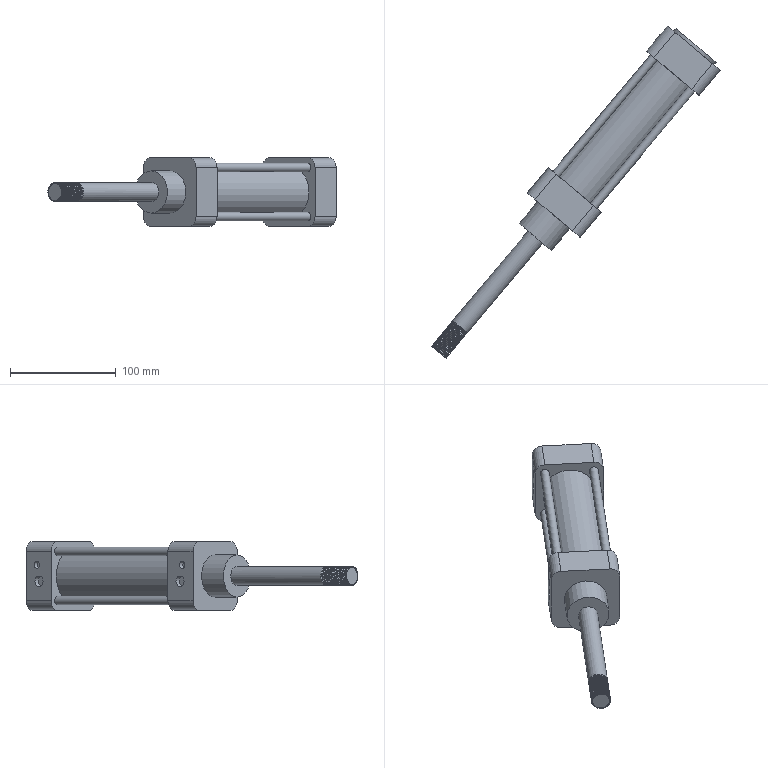Part | NX | features solid 2 | 1 solid | 71 faces | box 272.421 x 313.698 x 65 mm | volume 641095 mm3 | cylinder 45 | plane 24 | spline 2 | commonest cylinder face diameters 18 x21 18.5 x8 10 x6 8 x4 6.667 x2 50 x2